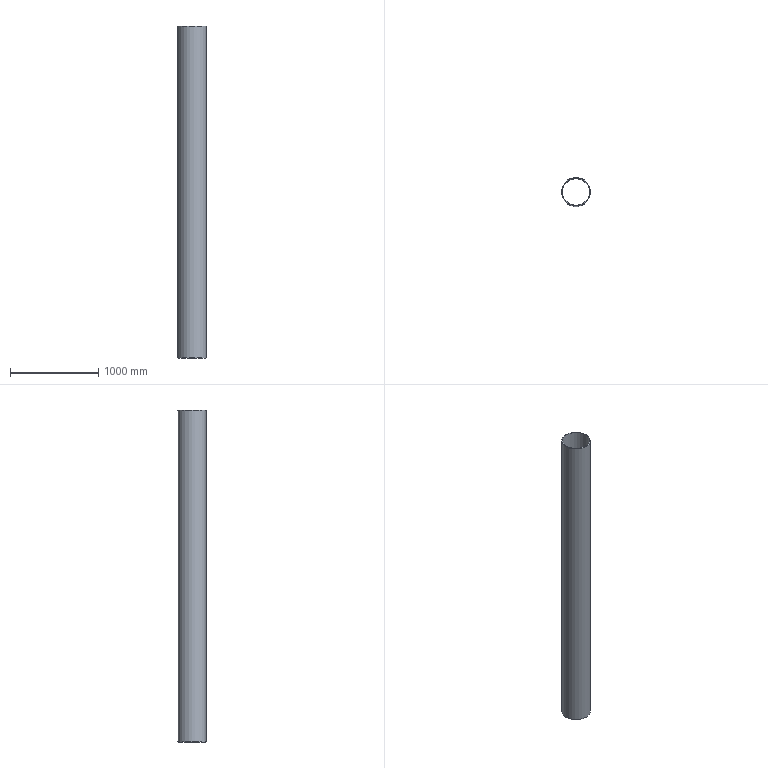Part | NX | features CHAMFER 1, CYLINDER 1, DATUM_CSYS 1, SHELL 1 | 1 solid | 6 faces | box 325 x 325 x 3759 mm | volume 29937295 mm3 | plane 2 | cylinder 2 | cone 2 | commonest cylinder face diameters 309 x1 325 x1
STEP:
#1=CARTESIAN_POINT('',(158.17,0.,3759.));
#2=VERTEX_POINT('',#1);
#3=CARTESIAN_POINT('',(0.,0.,3759.));
#4=DIRECTION('',(0.,0.,1.));
#5=DIRECTION('',(1.,0.,0.));
#6=AXIS2_PLACEMENT_3D('',#3,#4,#5);
#7=CIRCLE('',#6,158.17);
#8=EDGE_CURVE('',#2,#2,#7,.T.);
#9=ORIENTED_EDGE('',*,*,#8,.T.);
#10=EDGE_LOOP('',(#9));
#11=FACE_BOUND('',#10,.T.);
#12=CARTESIAN_POINT('',(154.5,0.,3759.));
#13=VERTEX_POINT('',#12);
#14=CARTESIAN_POINT('',(0.,0.,3759.));
#15=DIRECTION('',(0.,0.,1.));
#16=DIRECTION('',(1.,0.,0.));
#17=AXIS2_PLACEMENT_3D('',#14,#15,#16);
#18=CIRCLE('',#17,154.5);
#19=EDGE_CURVE('',#13,#13,#18,.F.);
#20=ORIENTED_EDGE('',*,*,#19,.T.);
#21=EDGE_LOOP('',(#20));
#22=FACE_BOUND('',#21,.T.);
#23=CARTESIAN_POINT('',(0.,0.,3759.));
#24=DIRECTION('',(0.,0.,1.));
#25=DIRECTION('',(1.,0.,0.));
#26=AXIS2_PLACEMENT_3D('',#23,#24,#25);
#27=PLANE('',#26);
#28=ADVANCED_FACE('',(#11,#22),#27,.T.);
#29=CARTESIAN_POINT('',(-158.17,0.,0.));
#30=VERTEX_POINT('',#29);
#31=CARTESIAN_POINT('',(0.,0.,0.));
#32=DIRECTION('',(0.,0.,-1.));
#33=DIRECTION('',(-1.,0.,0.));
#34=AXIS2_PLACEMENT_3D('',#31,#32,#33);
#35=CIRCLE('',#34,158.17);
#36=EDGE_CURVE('',#30,#30,#35,.T.);
#37=ORIENTED_EDGE('',*,*,#36,.T.);
#38=EDGE_LOOP('',(#37));
#39=FACE_BOUND('',#38,.T.);
#40=CARTESIAN_POINT('',(-154.5,0.,0.));
#41=VERTEX_POINT('',#40);
#42=CARTESIAN_POINT('',(0.,0.,0.));
#43=DIRECTION('',(0.,0.,-1.));
#44=DIRECTION('',(-1.,0.,0.));
#45=AXIS2_PLACEMENT_3D('',#42,#43,#44);
#46=CIRCLE('',#45,154.5);
#47=EDGE_CURVE('',#41,#41,#46,.F.);
#48=ORIENTED_EDGE('',*,*,#47,.T.);
#49=EDGE_LOOP('',(#48));
#50=FACE_BOUND('',#49,.T.);
#51=CARTESIAN_POINT('',(0.,0.,0.));
#52=DIRECTION('',(0.,0.,-1.));
#53=DIRECTION('',(-1.,0.,0.));
#54=AXIS2_PLACEMENT_3D('',#51,#52,#53);
#55=PLANE('',#54);
#56=ADVANCED_FACE('',(#39,#50),#55,.T.);
#57=CARTESIAN_POINT('',(-162.5,0.,2.5));
#58=VERTEX_POINT('',#57);
#59=CARTESIAN_POINT('',(0.,0.,2.5));
#60=DIRECTION('',(0.,0.,-1.));
#61=DIRECTION('',(-1.,0.,0.));
#62=AXIS2_PLACEMENT_3D('',#59,#60,#61);
#63=CIRCLE('',#62,162.5);
#64=EDGE_CURVE('',#58,#58,#63,.F.);
#65=ORIENTED_EDGE('',*,*,#64,.T.);
#66=EDGE_LOOP('',(#65));
#67=FACE_BOUND('',#66,.T.);
#68=CARTESIAN_POINT('',(162.5,0.,3756.5));
#69=VERTEX_POINT('',#68);
#70=CARTESIAN_POINT('',(0.,0.,3756.5));
#71=DIRECTION('',(0.,0.,1.));
#72=DIRECTION('',(1.,0.,0.));
#73=AXIS2_PLACEMENT_3D('',#70,#71,#72);
#74=CIRCLE('',#73,162.5);
#75=EDGE_CURVE('',#69,#69,#74,.F.);
#76=ORIENTED_EDGE('',*,*,#75,.T.);
#77=EDGE_LOOP('',(#76));
#78=FACE_BOUND('',#77,.T.);
#79=CARTESIAN_POINT('',(0.,0.,0.));
#80=DIRECTION('',(0.,0.,1.));
#81=DIRECTION('',(1.,0.,0.));
#82=AXIS2_PLACEMENT_3D('',#79,#80,#81);
#83=CYLINDRICAL_SURFACE('',#82,162.5);
#84=ADVANCED_FACE('',(#67,#78),#83,.T.);
#85=ORIENTED_EDGE('',*,*,#19,.F.);
#86=EDGE_LOOP('',(#85));
#87=FACE_BOUND('',#86,.T.);
#88=ORIENTED_EDGE('',*,*,#47,.F.);
#89=EDGE_LOOP('',(#88));
#90=FACE_BOUND('',#89,.T.);
#91=CARTESIAN_POINT('',(0.,0.,0.));
#92=DIRECTION('',(0.,0.,1.));
#93=DIRECTION('',(1.,0.,0.));
#94=AXIS2_PLACEMENT_3D('',#91,#92,#93);
#95=CYLINDRICAL_SURFACE('',#94,154.5);
#96=ADVANCED_FACE('',(#87,#90),#95,.F.);
#97=ORIENTED_EDGE('',*,*,#36,.F.);
#98=EDGE_LOOP('',(#97));
#99=FACE_BOUND('',#98,.T.);
#100=ORIENTED_EDGE('',*,*,#64,.F.);
#101=EDGE_LOOP('',(#100));
#102=FACE_BOUND('',#101,.T.);
#103=CARTESIAN_POINT('',(0.,0.,2.5));
#104=DIRECTION('',(0.,0.,1.));
#105=DIRECTION('',(1.,0.,0.));
#106=AXIS2_PLACEMENT_3D('',#103,#104,#105);
#107=CONICAL_SURFACE('',#106,162.5,1.047);
#108=ADVANCED_FACE('',(#99,#102),#107,.T.);
#109=ORIENTED_EDGE('',*,*,#8,.F.);
#110=EDGE_LOOP('',(#109));
#111=FACE_BOUND('',#110,.T.);
#112=ORIENTED_EDGE('',*,*,#75,.F.);
#113=EDGE_LOOP('',(#112));
#114=FACE_BOUND('',#113,.T.);
#115=CARTESIAN_POINT('',(0.,0.,3756.5));
#116=DIRECTION('',(0.,0.,-1.));
#117=DIRECTION('',(-1.,0.,0.));
#118=AXIS2_PLACEMENT_3D('',#115,#116,#117);
#119=CONICAL_SURFACE('',#118,162.5,1.047);
#120=ADVANCED_FACE('',(#111,#114),#119,.T.);
#121=CLOSED_SHELL('',(#28,#56,#84,#96,#108,#120));
#122=MANIFOLD_SOLID_BREP('',#121);
#123=(LENGTH_UNIT()NAMED_UNIT(*)SI_UNIT(.MILLI.,.METRE.));
#124=UNCERTAINTY_MEASURE_WITH_UNIT(LENGTH_MEASURE(0.00001),#123,'','');
#125=(NAMED_UNIT(*)PLANE_ANGLE_UNIT()SI_UNIT($,.RADIAN.));
#126=(NAMED_UNIT(*)SI_UNIT($,.STERADIAN.)SOLID_ANGLE_UNIT());
#127=(GEOMETRIC_REPRESENTATION_CONTEXT(3)GLOBAL_UNCERTAINTY_ASSIGNED_CONTEXT((#124))GLOBAL_UNIT_ASSIGNED_CONTEXT((#123,#125,#126))REPRESENTATION_CONTEXT('',''));
#128=ADVANCED_BREP_SHAPE_REPRESENTATION('',(#122),#127);